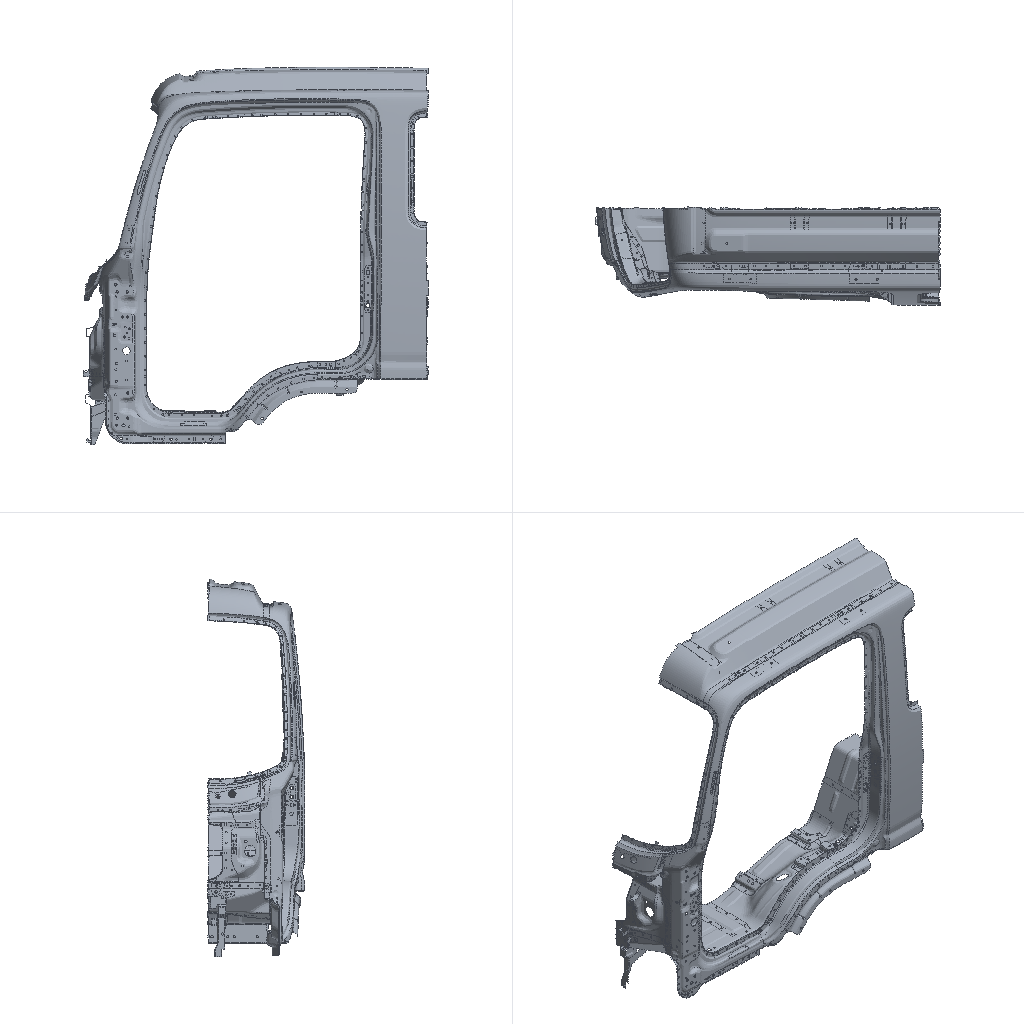Simulation study | nastran
Set-up summary:
category,name,step,type,value,unit,region
solver,nx_nastran
units,not stated in the deck,,not stated
analysis,deck,,static,static
analysis,solution,,SOL,101
load_step,SUBCASE 1,1,SUBCASE,SPC=2 LOAD=3
load_step,SUBCASE 2,2,SUBCASE,SPC=2 LOAD=4
load_step,SUBCASE 3,3,SUBCASE,SPC=2 LOAD=5
load_step,SUBCASE 4,4,SUBCASE,SPC=2 LOAD=9
load_step,SUBCASE 5,5,SUBCASE,SPC=2 LOAD=10
load_step,SUBCASE 6,6,SUBCASE,SPC=2 LOAD=11
load_step,SUBCASE 7,7,SUBCASE,SPC=2 LOAD=6
load_step,SUBCASE 8,8,SUBCASE,SPC=2 LOAD=7
load_step,SUBCASE 9,9,SUBCASE,SPC=2 LOAD=8
load_step,requested,,,9
mesh,nodes,,,64758
mesh,elements,,,58142
element_type,CHEXA,,unverified,496
element_type,CQUAD4,,shell,55421
element_type,CTRIA3,,shell,2721
load,load commands in deck,,count,9
bc,support commands in deck,,count,1506
check,setup vs results,,match,"every grid point's frame and coordinates and every element id; grid points of CHEXA, CQUAD4, CTRIA3 elements"
Nastran input file, long lists of numbers shortened:
$$------------------------------------------------------------------------------$
$$                                                                              $
$$ NASTRAN Input Deck Generated by HyperMesh Version  : 9.0b121                 $
$$ Generated using HyperMesh-Nastran Template Version : 9.0b121
$$                                                                              $
$$   Template:  general                                                         $
$$                                                                              $
$$------------------------------------------------------------------------------$
$$------------------------------------------------------------------------------$
$$                      Executive Control Cards                                 $
$$------------------------------------------------------------------------------$
SOL 101
CEND
$$------------------------------------------------------------------------------$
$$                      Case Control Cards                                      $
$$------------------------------------------------------------------------------$
  DISPLACEMENT = ALL
$
$HMNAME LOADSTEP               1"Fx"
SUBCASE       1
  LABEL=  Fx
  SPC =        2
  LOAD =        3
$
$HMNAME LOADSTEP               2"Fy"
SUBCASE       2
  LABEL=  Fy
  SPC =        2
  LOAD =        4
$
$HMNAME LOADSTEP               3"Fz"
SUBCASE       3
  LABEL=  Fz
  SPC =        2
  LOAD =        5
$
$HMNAME LOADSTEP               4"Rx"
SUBCASE       4
  LABEL=  Rx
  SPC =        2
  LOAD =        9
$
$HMNAME LOADSTEP               5"Ry"
SUBCASE       5
  LABEL=  Ry
  SPC =        2
  LOAD =       10
$
$HMNAME LOADSTEP               6"Rz"
SUBCASE       6
  LABEL=  Rz
  SPC =        2
  LOAD =       11
$
$HMNAME LOADSTEP               7"Ux"
SUBCASE       7
  LABEL=  Ux
  SPC =        2
  LOAD =        6
$
$HMNAME LOADSTEP               8"Uy"
SUBCASE       8
  LABEL=  Uy
  SPC =        2
  LOAD =        7
$
$HMNAME LOADSTEP               9"Uz"
SUBCASE       9
  LABEL=  Uz
  SPC =        2
  LOAD =        8
$$------------------------------------------------------------------------------$
$$                      Bulk Data Cards                                         $
$$------------------------------------------------------------------------------$
BEGIN BULK
PARAM,BAILOUT,-1
PARAM,POST,-1
$$
$$  GRID Data
$$
GRID          45        -598.898-842.1481708.803
GRID          46        -593.222-832.0261710.596
$ (64756 more lines like these left out)
$$
$$  SPOINT Data
$$
$$
$$------------------------------------------------------------------------------$
$$             Group Definitions                                                $
$$------------------------------------------------------------------------------$
$$
$$ RBE2 Elements - Multiple dependent nodes
$$
RBE2     103454084122189  123456  615912  615913  615914  615915  615916+
+         615917  615918  615919  615920  615921  615922  615923  615924+
+         615925  615926  615927  645474  645475  645476  645477  645478+
+         645479  645480  645481  645482  645483  645484  645485 3581857+
+        3581858 3581859 3581860 3581861 3581862 3581863 3581864 3581865+
+        3581866 3581867 3581868 3581957 3581958 3581959 3581960 3581961+
+        3581962 3581963 3581964 3581965 3581966 3581967 3581968 3581969+
+        3581970 3581971 3581972 3584087 3584088 3584089 3584090 3584091+
+        3584092 3584093 3584094 3584095 3584096 3584097 3584098 3584099+
+        3584100 3584101 3584102
RBE2     103454184122190  123456    1218    1220    1588    3981    4032+
+        3748844 3748845 3748846 3748847 3748848 3748849 3748850 3748851+
+        3748852 3748853 3749174 3749175 3749176 3749177 3749178 3749179+
+        3749180 3749181 3749182 3749183 3749184 3749271 3749272 3749273+
+        3749274 3749275 3749276 3749277 3749278 3749279 3749280 3749281+
+        3749282 3750713 3750733 3750752 3750753 3750754 3750758 3750759+
+        3750760 3750761 3751012 3751070 3751071 3751075 3751076 3751222+
+        3751223 3751224 3751269 3751270 3751271 3751275 3751279 3751283+
+        3751315 3751318 3751343 3751346 3751348 3751366 3751367 3751418+
+        3751450 3751451 3751452 3751454 3751455
RBE2     103454284122191  123456    1040   11942   12023  648196  648197+
+        3748717 3748718 3748719 3750118 3750129 3750130 3750606 3750607+
+        3750608 3750609 3750624 3750625 3750626 3750674 3750690 3750691+
+        3752922 3752926 3752927 3752928 3752929 3752930 3752931 3752933+
+        3752934 3752997 3753003 3753004 3754734 3754735 3754736 3754751+
+        3754752 3754776 3754777 3754778 3754779 3754780 3754781 3754782+
+        3754864 3754887 3754896 3754898 3754907 3754931 3754934 3754935+
+        3754940 3754941 3754944 3754945 3755004 3755008 3755009 3755210+
+
$
$HMMOVE 84022692
$        1034540THRU     1034542
$
$
$  RBE3 Elements
$
RBE3      326337         3755406  1234560.03889      123 37138720.025455+
+            123 37138710.370142     123 37138550.565513     123 3713854
RBE3      326338         3755407  1234560.623088     123 37138720.131026+
+            123 37138710.042722     123 37138550.203163     123 3713854
$ (7932 more lines like these left out)
$
$HMMOVE 57005012
$         326337THRU      326340  326342THRU      326349  326351THRU      326358
$         326360THRU      326367  326369THRU      326376  326378THRU      326385
$ (190 more lines like these left out)
CTRIA3    170731       3   87257   87311   87267
CTRIA3    170735       3   87254   87255   87266
$ (2719 more lines like these left out)
$
$HMMOVE       18
$         170731  170735  170737THRU      170738  170742  170748  170751  170762
$         195368  195423  198996THRU      198997
$ (360 more lines like these left out)
CQUAD4    170729       3   87267   87311   87259   87260
CQUAD4    170730       3   87264   87267   87260   87261
$ (55419 more lines like these left out)
$
$HMMOVE       18
$         170729THRU      170730  170732THRU      170734  170736  170739THRU
$         170741  170743THRU      170747  170749THRU      170750  170752THRU
$ (1295 more lines like these left out)
CHEXA     326341      10 3755406 3755409 3755408 3755407 3755410 3755413+
+        3755412 3755411
CHEXA     326350      10 3755415 3755416 3755417 3755418 3755419 3755420+
+        3755421 3755422
$ (988 more lines like these left out)
$
$HMMOVE 57005011
$         326341  326350  326359  326368  326377  326386  326953  326962  326971
$         326980  326989  326998  327007  327016  327619  327628  327637  327646
$ (220 more lines like these left out)
PSHELL         1       10.8            1               1
$
$HMNAME PROP                   2"120" 4
$HWCOLOR PROP                  2       3
PSHELL         2       11.2            1               1
$
$HMNAME PROP                   3"180" 4
$HWCOLOR PROP                  3       3
PSHELL         3       11.8            1               1
$
$HMNAME PROP                   4"100" 4
$HWCOLOR PROP                  4       3
PSHELL         4       11.0            1               1
$
$HMNAME PROP                   5"150" 4
$HWCOLOR PROP                  5       3
PSHELL         5       11.5            1               1
$
$HMNAME PROP                   6"250" 4
$HWCOLOR PROP                  6       3
PSHELL         6       12.5            1               1
$
$HMNAME PROP                   7"200" 4
$HWCOLOR PROP                  7       3
PSHELL         7       12.0            1               1
$$
$$  PSOLID Data
$
$HMNAME PROP                  10"spot" 5
$HWCOLOR PROP                 10       3
PSOLID        10       1
$$
$$------------------------------------------------------------------------------$
$$                      Material Definition Cards                               $
$$------------------------------------------------------------------------------$
$$--------------------------------------------------------------
$$ HYPERMESH TAGS
$$--------------------------------------------------------------
$$BEGIN TAGS
$$END TAGS
$$
$$  MAT1 Data
$
$HMNAME MAT                    1"steel" "MAT1"
$HWCOLOR MAT                   1       3
MAT1           1210000.0        0.3     1.60E-08
$$
$$
$$
$$------------------------------------------------------------------------------$
$ (61 more lines like these left out)
SPC            2   11391  1234560.0
SPC            2   11392  1234560.0
SPC            2   11455  1234560.0
SPC            2   11457  1234560.0
$ (1502 more lines like these left out)
$$
$$  FORCE Data
$$
FORCE          384122191       01.0     1000.0  0.0     0.0
FORCE          484122191       01.0     0.0     1000.0  0.0
FORCE          584122191       01.0     0.0     0.0     1000.0
FORCE          684122190       01.0     1000.0  0.0     0.0
FORCE          784122190       01.0     0.0     1000.0  0.0
FORCE          884122190       01.0     0.0     0.0     1000.0
FORCE          984122189       01.0     1000.0  0.0     0.0
FORCE         1084122189       01.0     0.0     1000.0  0.0
FORCE         1184122189       01.0     0.0     0.0     1000.0
$HMASSEM       1       3 REAR_FLOOR
$HMASSEM_IDS    5100990051000410510002105100111051001310510012105100141051001710
$HMASSEM_IDS    5100181251009310510042105100481151004311510054105100701051001021
$HMASSEM_IDS    510050105100991051009711
$HMASSEM      28       4 5300010
$HMASSEM_IDS          18      20      21      22      24      25      26
$HMASSEM 5700100       5 5700100
$HMASSEM_IDS    57001010570031105700201057004010
$HMASSEM 5400200       6 sidebody_R
$HMASSEM_IDS    54001220
$HMASSEM 5400100       7 sidebody_L
$HMASSEM_IDS    5400101054005010540070105400303054007020540030205400102054001030
$HMASSEM_IDS    5400111054001120540012105400301054005020
$
ENDDATA
Results summary:
result,analysis,,,static
result,last_loadstep,,,9
result,primary field,,,displacements
result,max displacement,,,1.249,model units